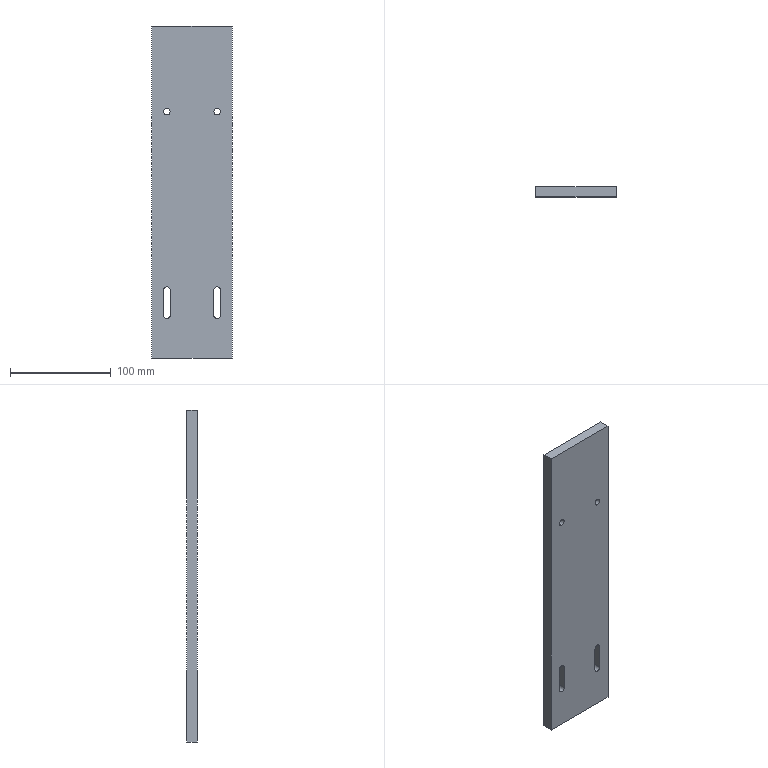Part | SolidWorks | features Extrusion 1, HoleWzd 1, ICE 1 | 1 solid | 20 faces | box 80 x 10 x 330 mm | volume 259332 mm3 | cylinder 10 | plane 10 | commonest cylinder face diameters 6.6 x10
STEP:
#1=CARTESIAN_POINT('',(-25.,0.,-94.2));
#2=VERTEX_POINT('',#1);
#3=CARTESIAN_POINT('',(-21.7,0.,-97.5));
#4=VERTEX_POINT('',#3);
#5=CARTESIAN_POINT('',(-25.,0.,-97.5));
#6=DIRECTION('',(0.,1.,0.));
#7=DIRECTION('',(0.,0.,1.));
#8=AXIS2_PLACEMENT_3D('',#5,#6,#7);
#9=CIRCLE('',#8,3.3);
#10=EDGE_CURVE('',#2,#4,#9,.T.);
#11=ORIENTED_EDGE('',*,*,#10,.F.);
#12=CARTESIAN_POINT('',(-25.,10.,-94.2));
#13=VERTEX_POINT('',#12);
#14=CARTESIAN_POINT('',(-25.,0.,-94.2));
#15=DIRECTION('',(0.,1.,0.));
#16=VECTOR('',#15,1000.);
#17=LINE('',#14,#16);
#18=EDGE_CURVE('',#2,#13,#17,.T.);
#19=ORIENTED_EDGE('',*,*,#18,.T.);
#20=CARTESIAN_POINT('',(-21.7,10.,-97.5));
#21=VERTEX_POINT('',#20);
#22=CARTESIAN_POINT('',(-25.,10.,-97.5));
#23=DIRECTION('',(0.,1.,0.));
#24=DIRECTION('',(0.,0.,1.));
#25=AXIS2_PLACEMENT_3D('',#22,#23,#24);
#26=CIRCLE('',#25,3.3);
#27=EDGE_CURVE('',#13,#21,#26,.T.);
#28=ORIENTED_EDGE('',*,*,#27,.T.);
#29=CARTESIAN_POINT('',(-21.7,0.,-97.5));
#30=DIRECTION('',(0.,1.,0.));
#31=VECTOR('',#30,1000.);
#32=LINE('',#29,#31);
#33=EDGE_CURVE('',#4,#21,#32,.T.);
#34=ORIENTED_EDGE('',*,*,#33,.F.);
#35=EDGE_LOOP('',(#11,#19,#28,#34));
#36=FACE_OUTER_BOUND('',#35,.T.);
#37=CARTESIAN_POINT('',(-25.,0.,-97.5));
#38=DIRECTION('',(0.,1.,0.));
#39=DIRECTION('',(0.,0.,1.));
#40=AXIS2_PLACEMENT_3D('',#37,#38,#39);
#41=CYLINDRICAL_SURFACE('',#40,3.3);
#42=ADVANCED_FACE('',(#36),#41,.F.);
#43=CARTESIAN_POINT('',(25.,0.,-94.2));
#44=VERTEX_POINT('',#43);
#45=CARTESIAN_POINT('',(28.3,0.,-97.5));
#46=VERTEX_POINT('',#45);
#47=CARTESIAN_POINT('',(25.,0.,-97.5));
#48=DIRECTION('',(0.,1.,0.));
#49=DIRECTION('',(0.,0.,1.));
#50=AXIS2_PLACEMENT_3D('',#47,#48,#49);
#51=CIRCLE('',#50,3.3);
#52=EDGE_CURVE('',#44,#46,#51,.T.);
#53=ORIENTED_EDGE('',*,*,#52,.F.);
#54=CARTESIAN_POINT('',(25.,10.,-94.2));
#55=VERTEX_POINT('',#54);
#56=CARTESIAN_POINT('',(25.,0.,-94.2));
#57=DIRECTION('',(0.,1.,0.));
#58=VECTOR('',#57,1000.);
#59=LINE('',#56,#58);
#60=EDGE_CURVE('',#44,#55,#59,.T.);
#61=ORIENTED_EDGE('',*,*,#60,.T.);
#62=CARTESIAN_POINT('',(28.3,10.,-97.5));
#63=VERTEX_POINT('',#62);
#64=CARTESIAN_POINT('',(25.,10.,-97.5));
#65=DIRECTION('',(0.,1.,0.));
#66=DIRECTION('',(0.,0.,1.));
#67=AXIS2_PLACEMENT_3D('',#64,#65,#66);
#68=CIRCLE('',#67,3.3);
#69=EDGE_CURVE('',#55,#63,#68,.T.);
#70=ORIENTED_EDGE('',*,*,#69,.T.);
#71=CARTESIAN_POINT('',(28.3,0.,-97.5));
#72=DIRECTION('',(0.,1.,0.));
#73=VECTOR('',#72,1000.);
#74=LINE('',#71,#73);
#75=EDGE_CURVE('',#46,#63,#74,.T.);
#76=ORIENTED_EDGE('',*,*,#75,.F.);
#77=EDGE_LOOP('',(#53,#61,#70,#76));
#78=FACE_OUTER_BOUND('',#77,.T.);
#79=CARTESIAN_POINT('',(25.,0.,-97.5));
#80=DIRECTION('',(0.,1.,0.));
#81=DIRECTION('',(0.,0.,1.));
#82=AXIS2_PLACEMENT_3D('',#79,#80,#81);
#83=CYLINDRICAL_SURFACE('',#82,3.3);
#84=ADVANCED_FACE('',(#78),#83,.F.);
#85=CARTESIAN_POINT('',(-25.,0.,76.7));
#86=VERTEX_POINT('',#85);
#87=CARTESIAN_POINT('',(-25.,0.,83.3));
#88=VERTEX_POINT('',#87);
#89=CARTESIAN_POINT('',(-25.,0.,80.));
#90=DIRECTION('',(0.,1.,0.));
#91=DIRECTION('',(0.,0.,1.));
#92=AXIS2_PLACEMENT_3D('',#89,#90,#91);
#93=CIRCLE('',#92,3.3);
#94=EDGE_CURVE('',#86,#88,#93,.T.);
#95=ORIENTED_EDGE('',*,*,#94,.F.);
#96=CARTESIAN_POINT('',(-25.,10.,76.7));
#97=VERTEX_POINT('',#96);
#98=CARTESIAN_POINT('',(-25.,10.,76.7));
#99=DIRECTION('',(0.,1.,0.));
#100=VECTOR('',#99,1000.);
#101=LINE('',#98,#100);
#102=EDGE_CURVE('',#86,#97,#101,.T.);
#103=ORIENTED_EDGE('',*,*,#102,.T.);
#104=CARTESIAN_POINT('',(-25.,10.,83.3));
#105=VERTEX_POINT('',#104);
#106=CARTESIAN_POINT('',(-25.,10.,80.));
#107=DIRECTION('',(0.,1.,0.));
#108=DIRECTION('',(0.,0.,1.));
#109=AXIS2_PLACEMENT_3D('',#106,#107,#108);
#110=CIRCLE('',#109,3.3);
#111=EDGE_CURVE('',#97,#105,#110,.T.);
#112=ORIENTED_EDGE('',*,*,#111,.T.);
#113=CARTESIAN_POINT('',(-25.,10.,83.3));
#114=DIRECTION('',(0.,1.,0.));
#115=VECTOR('',#114,1000.);
#116=LINE('',#113,#115);
#117=EDGE_CURVE('',#88,#105,#116,.T.);
#118=ORIENTED_EDGE('',*,*,#117,.F.);
#119=EDGE_LOOP('',(#95,#103,#112,#118));
#120=FACE_OUTER_BOUND('',#119,.T.);
#121=CARTESIAN_POINT('',(-25.,10.,80.));
#122=DIRECTION('',(0.,1.,0.));
#123=DIRECTION('',(0.,0.,1.));
#124=AXIS2_PLACEMENT_3D('',#121,#122,#123);
#125=CYLINDRICAL_SURFACE('',#124,3.3);
#126=ADVANCED_FACE('',(#120),#125,.F.);
#127=CARTESIAN_POINT('',(25.,0.,76.7));
#128=VERTEX_POINT('',#127);
#129=CARTESIAN_POINT('',(25.,0.,83.3));
#130=VERTEX_POINT('',#129);
#131=CARTESIAN_POINT('',(25.,0.,80.));
#132=DIRECTION('',(0.,1.,0.));
#133=DIRECTION('',(0.,0.,1.));
#134=AXIS2_PLACEMENT_3D('',#131,#132,#133);
#135=CIRCLE('',#134,3.3);
#136=EDGE_CURVE('',#128,#130,#135,.T.);
#137=ORIENTED_EDGE('',*,*,#136,.F.);
#138=CARTESIAN_POINT('',(25.,10.,76.7));
#139=VERTEX_POINT('',#138);
#140=CARTESIAN_POINT('',(25.,10.,76.7));
#141=DIRECTION('',(0.,1.,0.));
#142=VECTOR('',#141,1000.);
#143=LINE('',#140,#142);
#144=EDGE_CURVE('',#128,#139,#143,.T.);
#145=ORIENTED_EDGE('',*,*,#144,.T.);
#146=CARTESIAN_POINT('',(25.,10.,83.3));
#147=VERTEX_POINT('',#146);
#148=CARTESIAN_POINT('',(25.,10.,80.));
#149=DIRECTION('',(0.,1.,0.));
#150=DIRECTION('',(0.,0.,1.));
#151=AXIS2_PLACEMENT_3D('',#148,#149,#150);
#152=CIRCLE('',#151,3.3);
#153=EDGE_CURVE('',#139,#147,#152,.T.);
#154=ORIENTED_EDGE('',*,*,#153,.T.);
#155=CARTESIAN_POINT('',(25.,10.,83.3));
#156=DIRECTION('',(0.,1.,0.));
#157=VECTOR('',#156,1000.);
#158=LINE('',#155,#157);
#159=EDGE_CURVE('',#130,#147,#158,.T.);
#160=ORIENTED_EDGE('',*,*,#159,.F.);
#161=EDGE_LOOP('',(#137,#145,#154,#160));
#162=FACE_OUTER_BOUND('',#161,.T.);
#163=CARTESIAN_POINT('',(25.,10.,80.));
#164=DIRECTION('',(0.,1.,0.));
#165=DIRECTION('',(0.,0.,1.));
#166=AXIS2_PLACEMENT_3D('',#163,#164,#165);
#167=CYLINDRICAL_SURFACE('',#166,3.3);
#168=ADVANCED_FACE('',(#162),#167,.F.);
#169=CARTESIAN_POINT('',(40.,0.,165.));
#170=VERTEX_POINT('',#169);
#171=CARTESIAN_POINT('',(40.,0.,-165.));
#172=VERTEX_POINT('',#171);
#173=CARTESIAN_POINT('',(40.,0.,-165.));
#174=DIRECTION('',(0.,0.,-1.));
#175=VECTOR('',#174,1000.);
#176=LINE('',#173,#175);
#177=EDGE_CURVE('',#170,#172,#176,.T.);
#178=ORIENTED_EDGE('',*,*,#177,.T.);
#179=CARTESIAN_POINT('',(40.,10.,-165.));
#180=VERTEX_POINT('',#179);
#181=CARTESIAN_POINT('',(40.,10.,-165.));
#182=DIRECTION('',(0.,-1.,0.));
#183=VECTOR('',#182,1000.);
#184=LINE('',#181,#183);
#185=EDGE_CURVE('',#180,#172,#184,.T.);
#186=ORIENTED_EDGE('',*,*,#185,.F.);
#187=CARTESIAN_POINT('',(40.,10.,165.));
#188=VERTEX_POINT('',#187);
#189=CARTESIAN_POINT('',(40.,10.,-165.));
#190=DIRECTION('',(0.,0.,-1.));
#191=VECTOR('',#190,1000.);
#192=LINE('',#189,#191);
#193=EDGE_CURVE('',#188,#180,#192,.T.);
#194=ORIENTED_EDGE('',*,*,#193,.F.);
#195=CARTESIAN_POINT('',(40.,10.,165.));
#196=DIRECTION('',(0.,-1.,0.));
#197=VECTOR('',#196,1000.);
#198=LINE('',#195,#197);
#199=EDGE_CURVE('',#188,#170,#198,.T.);
#200=ORIENTED_EDGE('',*,*,#199,.T.);
#201=EDGE_LOOP('',(#178,#186,#194,#200));
#202=FACE_OUTER_BOUND('',#201,.T.);
#203=CARTESIAN_POINT('',(40.,10.,-165.));
#204=DIRECTION('',(-1.,0.,0.));
#205=DIRECTION('',(0.,0.,1.));
#206=AXIS2_PLACEMENT_3D('',#203,#204,#205);
#207=PLANE('',#206);
#208=ADVANCED_FACE('',(#202),#207,.F.);
#209=CARTESIAN_POINT('',(-40.,0.,-165.));
#210=VERTEX_POINT('',#209);
#211=CARTESIAN_POINT('',(-40.,0.,-165.));
#212=DIRECTION('',(-1.,0.,0.));
#213=VECTOR('',#212,1000.);
#214=LINE('',#211,#213);
#215=EDGE_CURVE('',#172,#210,#214,.T.);
#216=ORIENTED_EDGE('',*,*,#215,.T.);
#217=CARTESIAN_POINT('',(-40.,10.,-165.));
#218=VERTEX_POINT('',#217);
#219=CARTESIAN_POINT('',(-40.,10.,-165.));
#220=DIRECTION('',(0.,-1.,0.));
#221=VECTOR('',#220,1000.);
#222=LINE('',#219,#221);
#223=EDGE_CURVE('',#218,#210,#222,.T.);
#224=ORIENTED_EDGE('',*,*,#223,.F.);
#225=CARTESIAN_POINT('',(-40.,10.,-165.));
#226=DIRECTION('',(-1.,0.,0.));
#227=VECTOR('',#226,1000.);
#228=LINE('',#225,#227);
#229=EDGE_CURVE('',#180,#218,#228,.T.);
#230=ORIENTED_EDGE('',*,*,#229,.F.);
#231=ORIENTED_EDGE('',*,*,#185,.T.);
#232=EDGE_LOOP('',(#216,#224,#230,#231));
#233=FACE_OUTER_BOUND('',#232,.T.);
#234=CARTESIAN_POINT('',(-40.,10.,-165.));
#235=DIRECTION('',(0.,0.,1.));
#236=DIRECTION('',(1.,0.,0.));
#237=AXIS2_PLACEMENT_3D('',#234,#235,#236);
#238=PLANE('',#237);
#239=ADVANCED_FACE('',(#233),#238,.F.);
#240=CARTESIAN_POINT('',(-40.,0.,165.));
#241=VERTEX_POINT('',#240);
#242=CARTESIAN_POINT('',(-40.,0.,-165.));
#243=DIRECTION('',(0.,0.,1.));
#244=VECTOR('',#243,1000.);
#245=LINE('',#242,#244);
#246=EDGE_CURVE('',#210,#241,#245,.T.);
#247=ORIENTED_EDGE('',*,*,#246,.T.);
#248=CARTESIAN_POINT('',(-40.,10.,165.));
#249=VERTEX_POINT('',#248);
#250=CARTESIAN_POINT('',(-40.,10.,165.));
#251=DIRECTION('',(0.,-1.,0.));
#252=VECTOR('',#251,1000.);
#253=LINE('',#250,#252);
#254=EDGE_CURVE('',#249,#241,#253,.T.);
#255=ORIENTED_EDGE('',*,*,#254,.F.);
#256=CARTESIAN_POINT('',(-40.,10.,-165.));
#257=DIRECTION('',(0.,0.,1.));
#258=VECTOR('',#257,1000.);
#259=LINE('',#256,#258);
#260=EDGE_CURVE('',#218,#249,#259,.T.);
#261=ORIENTED_EDGE('',*,*,#260,.F.);
#262=ORIENTED_EDGE('',*,*,#223,.T.);
#263=EDGE_LOOP('',(#247,#255,#261,#262));
#264=FACE_OUTER_BOUND('',#263,.T.);
#265=CARTESIAN_POINT('',(-40.,10.,-165.));
#266=DIRECTION('',(1.,0.,0.));
#267=DIRECTION('',(0.,0.,-1.));
#268=AXIS2_PLACEMENT_3D('',#265,#266,#267);
#269=PLANE('',#268);
#270=ADVANCED_FACE('',(#264),#269,.F.);
#271=CARTESIAN_POINT('',(-40.,0.,165.));
#272=DIRECTION('',(1.,0.,0.));
#273=VECTOR('',#272,1000.);
#274=LINE('',#271,#273);
#275=EDGE_CURVE('',#241,#170,#274,.T.);
#276=ORIENTED_EDGE('',*,*,#275,.T.);
#277=ORIENTED_EDGE('',*,*,#199,.F.);
#278=CARTESIAN_POINT('',(-40.,10.,165.));
#279=DIRECTION('',(1.,0.,0.));
#280=VECTOR('',#279,1000.);
#281=LINE('',#278,#280);
#282=EDGE_CURVE('',#249,#188,#281,.T.);
#283=ORIENTED_EDGE('',*,*,#282,.F.);
#284=ORIENTED_EDGE('',*,*,#254,.T.);
#285=EDGE_LOOP('',(#276,#277,#283,#284));
#286=FACE_OUTER_BOUND('',#285,.T.);
#287=CARTESIAN_POINT('',(-40.,10.,165.));
#288=DIRECTION('',(0.,0.,-1.));
#289=DIRECTION('',(-1.,0.,0.));
#290=AXIS2_PLACEMENT_3D('',#287,#288,#289);
#291=PLANE('',#290);
#292=ADVANCED_FACE('',(#286),#291,.F.);
#293=CARTESIAN_POINT('',(-28.3,10.,-97.5));
#294=VERTEX_POINT('',#293);
#295=CARTESIAN_POINT('',(-25.,10.,-97.5));
#296=DIRECTION('',(0.,1.,0.));
#297=DIRECTION('',(0.,0.,1.));
#298=AXIS2_PLACEMENT_3D('',#295,#296,#297);
#299=CIRCLE('',#298,3.3);
#300=EDGE_CURVE('',#294,#13,#299,.T.);
#301=ORIENTED_EDGE('',*,*,#300,.F.);
#302=CARTESIAN_POINT('',(-28.3,10.,-122.5));
#303=VERTEX_POINT('',#302);
#304=CARTESIAN_POINT('',(-28.3,10.,-97.5));
#305=DIRECTION('',(0.,0.,1.));
#306=VECTOR('',#305,1000.);
#307=LINE('',#304,#306);
#308=EDGE_CURVE('',#303,#294,#307,.T.);
#309=ORIENTED_EDGE('',*,*,#308,.F.);
#310=CARTESIAN_POINT('',(-21.7,10.,-122.5));
#311=VERTEX_POINT('',#310);
#312=CARTESIAN_POINT('',(-25.,10.,-122.5));
#313=DIRECTION('',(0.,1.,0.));
#314=DIRECTION('',(0.,0.,1.));
#315=AXIS2_PLACEMENT_3D('',#312,#313,#314);
#316=CIRCLE('',#315,3.3);
#317=EDGE_CURVE('',#311,#303,#316,.T.);
#318=ORIENTED_EDGE('',*,*,#317,.F.);
#319=CARTESIAN_POINT('',(-21.7,10.,-97.5));
#320=DIRECTION('',(0.,0.,-1.));
#321=VECTOR('',#320,1000.);
#322=LINE('',#319,#321);
#323=EDGE_CURVE('',#21,#311,#322,.T.);
#324=ORIENTED_EDGE('',*,*,#323,.F.);
#325=ORIENTED_EDGE('',*,*,#27,.F.);
#326=EDGE_LOOP('',(#301,#309,#318,#324,#325));
#327=FACE_BOUND('',#326,.T.);
#328=CARTESIAN_POINT('',(21.7,10.,-97.5));
#329=VERTEX_POINT('',#328);
#330=CARTESIAN_POINT('',(25.,10.,-97.5));
#331=DIRECTION('',(0.,1.,0.));
#332=DIRECTION('',(0.,0.,1.));
#333=AXIS2_PLACEMENT_3D('',#330,#331,#332);
#334=CIRCLE('',#333,3.3);
#335=EDGE_CURVE('',#329,#55,#334,.T.);
#336=ORIENTED_EDGE('',*,*,#335,.F.);
#337=CARTESIAN_POINT('',(21.7,10.,-122.5));
#338=VERTEX_POINT('',#337);
#339=CARTESIAN_POINT('',(21.7,10.,-97.5));
#340=DIRECTION('',(0.,0.,1.));
#341=VECTOR('',#340,1000.);
#342=LINE('',#339,#341);
#343=EDGE_CURVE('',#338,#329,#342,.T.);
#344=ORIENTED_EDGE('',*,*,#343,.F.);
#345=CARTESIAN_POINT('',(28.3,10.,-122.5));
#346=VERTEX_POINT('',#345);
#347=CARTESIAN_POINT('',(25.,10.,-122.5));
#348=DIRECTION('',(0.,1.,0.));
#349=DIRECTION('',(0.,0.,1.));
#350=AXIS2_PLACEMENT_3D('',#347,#348,#349);
#351=CIRCLE('',#350,3.3);
#352=EDGE_CURVE('',#346,#338,#351,.T.);
#353=ORIENTED_EDGE('',*,*,#352,.F.);
#354=CARTESIAN_POINT('',(28.3,10.,-97.5));
#355=DIRECTION('',(0.,0.,-1.));
#356=VECTOR('',#355,1000.);
#357=LINE('',#354,#356);
#358=EDGE_CURVE('',#63,#346,#357,.T.);
#359=ORIENTED_EDGE('',*,*,#358,.F.);
#360=ORIENTED_EDGE('',*,*,#69,.F.);
#361=EDGE_LOOP('',(#336,#344,#353,#359,#360));
#362=FACE_BOUND('',#361,.T.);
#363=CARTESIAN_POINT('',(-25.,10.,80.));
#364=DIRECTION('',(0.,1.,0.));
#365=DIRECTION('',(0.,0.,1.));
#366=AXIS2_PLACEMENT_3D('',#363,#364,#365);
#367=CIRCLE('',#366,3.3);
#368=EDGE_CURVE('',#105,#97,#367,.T.);
#369=ORIENTED_EDGE('',*,*,#368,.F.);
#370=ORIENTED_EDGE('',*,*,#111,.F.);
#371=EDGE_LOOP('',(#369,#370));
#372=FACE_BOUND('',#371,.T.);
#373=CARTESIAN_POINT('',(25.,10.,80.));
#374=DIRECTION('',(0.,1.,0.));
#375=DIRECTION('',(0.,0.,1.));
#376=AXIS2_PLACEMENT_3D('',#373,#374,#375);
#377=CIRCLE('',#376,3.3);
#378=EDGE_CURVE('',#147,#139,#377,.T.);
#379=ORIENTED_EDGE('',*,*,#378,.F.);
#380=ORIENTED_EDGE('',*,*,#153,.F.);
#381=EDGE_LOOP('',(#379,#380));
#382=FACE_BOUND('',#381,.T.);
#383=ORIENTED_EDGE('',*,*,#193,.T.);
#384=ORIENTED_EDGE('',*,*,#229,.T.);
#385=ORIENTED_EDGE('',*,*,#260,.T.);
#386=ORIENTED_EDGE('',*,*,#282,.T.);
#387=EDGE_LOOP('',(#383,#384,#385,#386));
#388=FACE_OUTER_BOUND('',#387,.T.);
#389=CARTESIAN_POINT('',(0.,10.,0.));
#390=DIRECTION('',(0.,1.,0.));
#391=DIRECTION('',(0.,0.,1.));
#392=AXIS2_PLACEMENT_3D('',#389,#390,#391);
#393=PLANE('',#392);
#394=ADVANCED_FACE('',(#327,#362,#372,#382,#388),#393,.T.);
#395=CARTESIAN_POINT('',(-28.3,0.,-122.5));
#396=VERTEX_POINT('',#395);
#397=CARTESIAN_POINT('',(-28.3,0.,-97.5));
#398=VERTEX_POINT('',#397);
#399=CARTESIAN_POINT('',(-28.3,0.,-97.5));
#400=DIRECTION('',(0.,0.,1.));
#401=VECTOR('',#400,1000.);
#402=LINE('',#399,#401);
#403=EDGE_CURVE('',#396,#398,#402,.T.);
#404=ORIENTED_EDGE('',*,*,#403,.T.);
#405=CARTESIAN_POINT('',(-25.,0.,-97.5));
#406=DIRECTION('',(0.,1.,0.));
#407=DIRECTION('',(0.,0.,1.));
#408=AXIS2_PLACEMENT_3D('',#405,#406,#407);
#409=CIRCLE('',#408,3.3);
#410=EDGE_CURVE('',#398,#2,#409,.T.);
#411=ORIENTED_EDGE('',*,*,#410,.T.);
#412=ORIENTED_EDGE('',*,*,#10,.T.);
#413=CARTESIAN_POINT('',(-21.7,0.,-122.5));
#414=VERTEX_POINT('',#413);
#415=CARTESIAN_POINT('',(-21.7,0.,-97.5));
#416=DIRECTION('',(0.,0.,-1.));
#417=VECTOR('',#416,1000.);
#418=LINE('',#415,#417);
#419=EDGE_CURVE('',#4,#414,#418,.T.);
#420=ORIENTED_EDGE('',*,*,#419,.T.);
#421=CARTESIAN_POINT('',(-25.,0.,-122.5));
#422=DIRECTION('',(0.,1.,0.));
#423=DIRECTION('',(0.,0.,1.));
#424=AXIS2_PLACEMENT_3D('',#421,#422,#423);
#425=CIRCLE('',#424,3.3);
#426=EDGE_CURVE('',#414,#396,#425,.T.);
#427=ORIENTED_EDGE('',*,*,#426,.T.);
#428=EDGE_LOOP('',(#404,#411,#412,#420,#427));
#429=FACE_BOUND('',#428,.T.);
#430=CARTESIAN_POINT('',(21.7,0.,-122.5));
#431=VERTEX_POINT('',#430);
#432=CARTESIAN_POINT('',(21.7,0.,-97.5));
#433=VERTEX_POINT('',#432);
#434=CARTESIAN_POINT('',(21.7,0.,-97.5));
#435=DIRECTION('',(0.,0.,1.));
#436=VECTOR('',#435,1000.);
#437=LINE('',#434,#436);
#438=EDGE_CURVE('',#431,#433,#437,.T.);
#439=ORIENTED_EDGE('',*,*,#438,.T.);
#440=CARTESIAN_POINT('',(25.,0.,-97.5));
#441=DIRECTION('',(0.,1.,0.));
#442=DIRECTION('',(0.,0.,1.));
#443=AXIS2_PLACEMENT_3D('',#440,#441,#442);
#444=CIRCLE('',#443,3.3);
#445=EDGE_CURVE('',#433,#44,#444,.T.);
#446=ORIENTED_EDGE('',*,*,#445,.T.);
#447=ORIENTED_EDGE('',*,*,#52,.T.);
#448=CARTESIAN_POINT('',(28.3,0.,-122.5));
#449=VERTEX_POINT('',#448);
#450=CARTESIAN_POINT('',(28.3,0.,-97.5));
#451=DIRECTION('',(0.,0.,-1.));
#452=VECTOR('',#451,1000.);
#453=LINE('',#450,#452);
#454=EDGE_CURVE('',#46,#449,#453,.T.);
#455=ORIENTED_EDGE('',*,*,#454,.T.);
#456=CARTESIAN_POINT('',(25.,0.,-122.5));
#457=DIRECTION('',(0.,1.,0.));
#458=DIRECTION('',(0.,0.,1.));
#459=AXIS2_PLACEMENT_3D('',#456,#457,#458);
#460=CIRCLE('',#459,3.3);
#461=EDGE_CURVE('',#449,#431,#460,.T.);
#462=ORIENTED_EDGE('',*,*,#461,.T.);
#463=EDGE_LOOP('',(#439,#446,#447,#455,#462));
#464=FACE_BOUND('',#463,.T.);
#465=CARTESIAN_POINT('',(-25.,0.,80.));
#466=DIRECTION('',(0.,1.,0.));
#467=DIRECTION('',(0.,0.,1.));
#468=AXIS2_PLACEMENT_3D('',#465,#466,#467);
#469=CIRCLE('',#468,3.3);
#470=EDGE_CURVE('',#88,#86,#469,.T.);
#471=ORIENTED_EDGE('',*,*,#470,.T.);
#472=ORIENTED_EDGE('',*,*,#94,.T.);
#473=EDGE_LOOP('',(#471,#472));
#474=FACE_BOUND('',#473,.T.);
#475=CARTESIAN_POINT('',(25.,0.,80.));
#476=DIRECTION('',(0.,1.,0.));
#477=DIRECTION('',(0.,0.,1.));
#478=AXIS2_PLACEMENT_3D('',#475,#476,#477);
#479=CIRCLE('',#478,3.3);
#480=EDGE_CURVE('',#130,#128,#479,.T.);
#481=ORIENTED_EDGE('',*,*,#480,.T.);
#482=ORIENTED_EDGE('',*,*,#136,.T.);
#483=EDGE_LOOP('',(#481,#482));
#484=FACE_BOUND('',#483,.T.);
#485=ORIENTED_EDGE('',*,*,#177,.F.);
#486=ORIENTED_EDGE('',*,*,#275,.F.);
#487=ORIENTED_EDGE('',*,*,#246,.F.);
#488=ORIENTED_EDGE('',*,*,#215,.F.);
#489=EDGE_LOOP('',(#485,#486,#487,#488));
#490=FACE_OUTER_BOUND('',#489,.T.);
#491=CARTESIAN_POINT('',(0.,0.,0.));
#492=DIRECTION('',(0.,1.,0.));
#493=DIRECTION('',(0.,0.,1.));
#494=AXIS2_PLACEMENT_3D('',#491,#492,#493);
#495=PLANE('',#494);
#496=ADVANCED_FACE('',(#429,#464,#474,#484,#490),#495,.F.);
#497=ORIENTED_EDGE('',*,*,#144,.F.);
#498=ORIENTED_EDGE('',*,*,#480,.F.);
#499=ORIENTED_EDGE('',*,*,#159,.T.);
#500=ORIENTED_EDGE('',*,*,#378,.T.);
#501=EDGE_LOOP('',(#497,#498,#499,#500));
#502=FACE_OUTER_BOUND('',#501,.T.);
#503=CARTESIAN_POINT('',(25.,10.,80.));
#504=DIRECTION('',(0.,1.,0.));
#505=DIRECTION('',(0.,0.,1.));
#506=AXIS2_PLACEMENT_3D('',#503,#504,#505);
#507=CYLINDRICAL_SURFACE('',#506,3.3);
#508=ADVANCED_FACE('',(#502),#507,.F.);
#509=ORIENTED_EDGE('',*,*,#102,.F.);
#510=ORIENTED_EDGE('',*,*,#470,.F.);
#511=ORIENTED_EDGE('',*,*,#117,.T.);
#512=ORIENTED_EDGE('',*,*,#368,.T.);
#513=EDGE_LOOP('',(#509,#510,#511,#512));
#514=FACE_OUTER_BOUND('',#513,.T.);
#515=CARTESIAN_POINT('',(-25.,10.,80.));
#516=DIRECTION('',(0.,1.,0.));
#517=DIRECTION('',(0.,0.,1.));
#518=AXIS2_PLACEMENT_3D('',#515,#516,#517);
#519=CYLINDRICAL_SURFACE('',#518,3.3);
#520=ADVANCED_FACE('',(#514),#519,.F.);
#521=ORIENTED_EDGE('',*,*,#60,.F.);
#522=ORIENTED_EDGE('',*,*,#445,.F.);
#523=CARTESIAN_POINT('',(21.7,0.,-97.5));
#524=DIRECTION('',(0.,1.,0.));
#525=VECTOR('',#524,1000.);
#526=LINE('',#523,#525);
#527=EDGE_CURVE('',#433,#329,#526,.T.);
#528=ORIENTED_EDGE('',*,*,#527,.T.);
#529=ORIENTED_EDGE('',*,*,#335,.T.);
#530=EDGE_LOOP('',(#521,#522,#528,#529));
#531=FACE_OUTER_BOUND('',#530,.T.);
#532=CARTESIAN_POINT('',(25.,0.,-97.5));
#533=DIRECTION('',(0.,1.,0.));
#534=DIRECTION('',(0.,0.,1.));
#535=AXIS2_PLACEMENT_3D('',#532,#533,#534);
#536=CYLINDRICAL_SURFACE('',#535,3.3);
#537=ADVANCED_FACE('',(#531),#536,.F.);
#538=ORIENTED_EDGE('',*,*,#343,.T.);
#539=ORIENTED_EDGE('',*,*,#527,.F.);
#540=ORIENTED_EDGE('',*,*,#438,.F.);
#541=CARTESIAN_POINT('',(21.7,0.,-122.5));
#542=DIRECTION('',(0.,1.,0.));
#543=VECTOR('',#542,1000.);
#544=LINE('',#541,#543);
#545=EDGE_CURVE('',#431,#338,#544,.T.);
#546=ORIENTED_EDGE('',*,*,#545,.T.);
#547=EDGE_LOOP('',(#538,#539,#540,#546));
#548=FACE_OUTER_BOUND('',#547,.T.);
#549=CARTESIAN_POINT('',(21.7,0.,-97.5));
#550=DIRECTION('',(-1.,0.,0.));
#551=DIRECTION('',(0.,0.,1.));
#552=AXIS2_PLACEMENT_3D('',#549,#550,#551);
#553=PLANE('',#552);
#554=ADVANCED_FACE('',(#548),#553,.F.);
#555=ORIENTED_EDGE('',*,*,#352,.T.);
#556=ORIENTED_EDGE('',*,*,#545,.F.);
#557=ORIENTED_EDGE('',*,*,#461,.F.);
#558=CARTESIAN_POINT('',(28.3,0.,-122.5));
#559=DIRECTION('',(0.,1.,0.));
#560=VECTOR('',#559,1000.);
#561=LINE('',#558,#560);
#562=EDGE_CURVE('',#449,#346,#561,.T.);
#563=ORIENTED_EDGE('',*,*,#562,.T.);
#564=EDGE_LOOP('',(#555,#556,#557,#563));
#565=FACE_OUTER_BOUND('',#564,.T.);
#566=CARTESIAN_POINT('',(25.,0.,-122.5));
#567=DIRECTION('',(0.,1.,0.));
#568=DIRECTION('',(0.,0.,1.));
#569=AXIS2_PLACEMENT_3D('',#566,#567,#568);
#570=CYLINDRICAL_SURFACE('',#569,3.3);
#571=ADVANCED_FACE('',(#565),#570,.F.);
#572=ORIENTED_EDGE('',*,*,#358,.T.);
#573=ORIENTED_EDGE('',*,*,#562,.F.);
#574=ORIENTED_EDGE('',*,*,#454,.F.);
#575=ORIENTED_EDGE('',*,*,#75,.T.);
#576=EDGE_LOOP('',(#572,#573,#574,#575));
#577=FACE_OUTER_BOUND('',#576,.T.);
#578=CARTESIAN_POINT('',(28.3,0.,-97.5));
#579=DIRECTION('',(1.,0.,0.));
#580=DIRECTION('',(0.,0.,-1.));
#581=AXIS2_PLACEMENT_3D('',#578,#579,#580);
#582=PLANE('',#581);
#583=ADVANCED_FACE('',(#577),#582,.F.);
#584=ORIENTED_EDGE('',*,*,#18,.F.);
#585=ORIENTED_EDGE('',*,*,#410,.F.);
#586=CARTESIAN_POINT('',(-28.3,0.,-97.5));
#587=DIRECTION('',(0.,1.,0.));
#588=VECTOR('',#587,1000.);
#589=LINE('',#586,#588);
#590=EDGE_CURVE('',#398,#294,#589,.T.);
#591=ORIENTED_EDGE('',*,*,#590,.T.);
#592=ORIENTED_EDGE('',*,*,#300,.T.);
#593=EDGE_LOOP('',(#584,#585,#591,#592));
#594=FACE_OUTER_BOUND('',#593,.T.);
#595=CARTESIAN_POINT('',(-25.,0.,-97.5));
#596=DIRECTION('',(0.,1.,0.));
#597=DIRECTION('',(0.,0.,1.));
#598=AXIS2_PLACEMENT_3D('',#595,#596,#597);
#599=CYLINDRICAL_SURFACE('',#598,3.3);
#600=ADVANCED_FACE('',(#594),#599,.F.);
#601=ORIENTED_EDGE('',*,*,#308,.T.);
#602=ORIENTED_EDGE('',*,*,#590,.F.);
#603=ORIENTED_EDGE('',*,*,#403,.F.);
#604=CARTESIAN_POINT('',(-28.3,0.,-122.5));
#605=DIRECTION('',(0.,1.,0.));
#606=VECTOR('',#605,1000.);
#607=LINE('',#604,#606);
#608=EDGE_CURVE('',#396,#303,#607,.T.);
#609=ORIENTED_EDGE('',*,*,#608,.T.);
#610=EDGE_LOOP('',(#601,#602,#603,#609));
#611=FACE_OUTER_BOUND('',#610,.T.);
#612=CARTESIAN_POINT('',(-28.3,0.,-97.5));
#613=DIRECTION('',(-1.,0.,0.));
#614=DIRECTION('',(0.,0.,1.));
#615=AXIS2_PLACEMENT_3D('',#612,#613,#614);
#616=PLANE('',#615);
#617=ADVANCED_FACE('',(#611),#616,.F.);
#618=ORIENTED_EDGE('',*,*,#317,.T.);
#619=ORIENTED_EDGE('',*,*,#608,.F.);
#620=ORIENTED_EDGE('',*,*,#426,.F.);
#621=CARTESIAN_POINT('',(-21.7,0.,-122.5));
#622=DIRECTION('',(0.,1.,0.));
#623=VECTOR('',#622,1000.);
#624=LINE('',#621,#623);
#625=EDGE_CURVE('',#414,#311,#624,.T.);
#626=ORIENTED_EDGE('',*,*,#625,.T.);
#627=EDGE_LOOP('',(#618,#619,#620,#626));
#628=FACE_OUTER_BOUND('',#627,.T.);
#629=CARTESIAN_POINT('',(-25.,0.,-122.5));
#630=DIRECTION('',(0.,1.,0.));
#631=DIRECTION('',(0.,0.,1.));
#632=AXIS2_PLACEMENT_3D('',#629,#630,#631);
#633=CYLINDRICAL_SURFACE('',#632,3.3);
#634=ADVANCED_FACE('',(#628),#633,.F.);
#635=ORIENTED_EDGE('',*,*,#323,.T.);
#636=ORIENTED_EDGE('',*,*,#625,.F.);
#637=ORIENTED_EDGE('',*,*,#419,.F.);
#638=ORIENTED_EDGE('',*,*,#33,.T.);
#639=EDGE_LOOP('',(#635,#636,#637,#638));
#640=FACE_OUTER_BOUND('',#639,.T.);
#641=CARTESIAN_POINT('',(-21.7,0.,-97.5));
#642=DIRECTION('',(1.,0.,0.));
#643=DIRECTION('',(0.,0.,-1.));
#644=AXIS2_PLACEMENT_3D('',#641,#642,#643);
#645=PLANE('',#644);
#646=ADVANCED_FACE('',(#640),#645,.F.);
#647=CLOSED_SHELL('',(#42,#84,#126,#168,#208,#239,#270,#292,#394,#496,#508,#520,#537,#554,#571,#583,#600,#617,#634,#646));
#648=MANIFOLD_SOLID_BREP('',#647);
#649=CARTESIAN_POINT('',(0.,0.,0.));
#650=DIRECTION('',(0.,0.,1.));
#651=DIRECTION('',(1.,0.,0.));
#652=AXIS2_PLACEMENT_3D('',#649,#650,#651);
#653=(LENGTH_UNIT()NAMED_UNIT(*)SI_UNIT(.MILLI.,.METRE.));
#654=UNCERTAINTY_MEASURE_WITH_UNIT(LENGTH_MEASURE(0.00001),#653,'','');
#655=(NAMED_UNIT(*)PLANE_ANGLE_UNIT()SI_UNIT($,.RADIAN.));
#656=(NAMED_UNIT(*)SI_UNIT($,.STERADIAN.)SOLID_ANGLE_UNIT());
#657=(GEOMETRIC_REPRESENTATION_CONTEXT(3)GLOBAL_UNCERTAINTY_ASSIGNED_CONTEXT((#654))GLOBAL_UNIT_ASSIGNED_CONTEXT((#653,#655,#656))REPRESENTATION_CONTEXT('',''));
#658=ADVANCED_BREP_SHAPE_REPRESENTATION('',(#648,#652),#657);